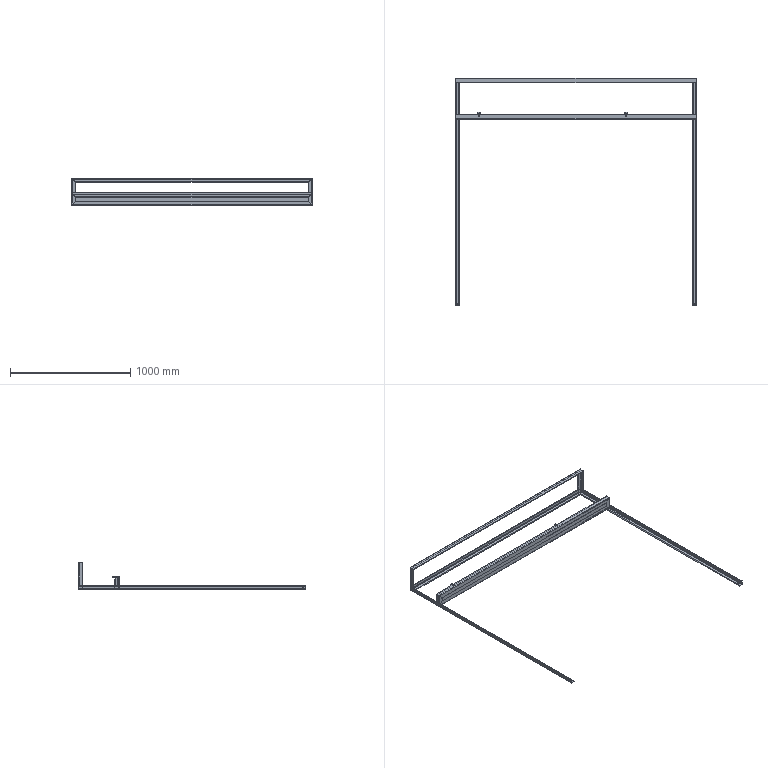Part | SolidWorks | features ICE 6, WeldMemberFeat 3, WeldmentFeature 1 | 12 solids | 130 faces | box 2010 x 1894 x 230 mm | volume 4743265 mm3 | plane 86 | cylinder 44 | commonest cylinder face diameters 10 x34 9 x6 7 x4